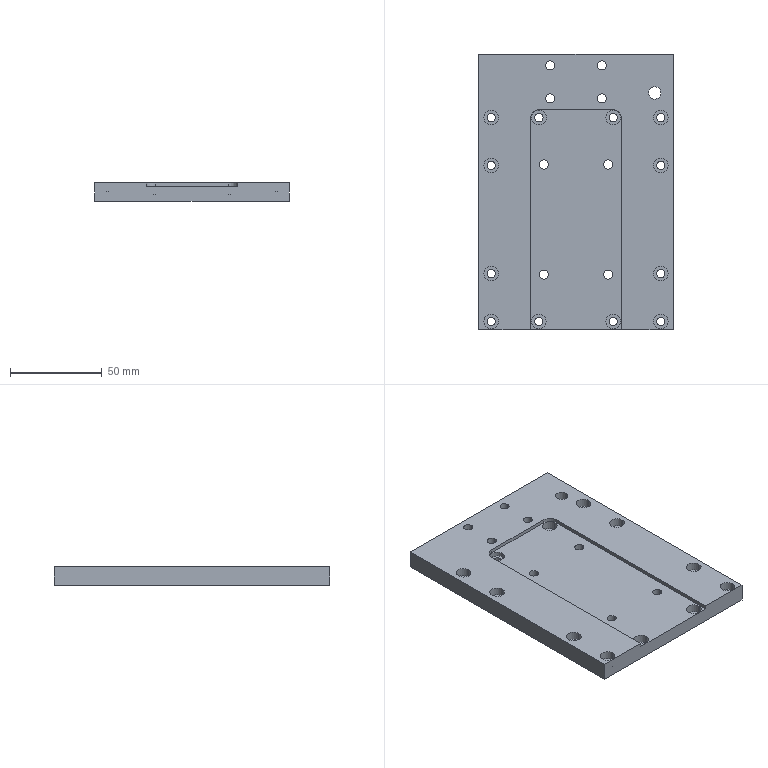Part | STEP file | X77-04014 | 1 solid | 90 faces | box 105.8 x 150 x 10 mm | volume 141335 mm3 | cylinder 68 | plane 22 | commonest cylinder face diameters 4.5 x24 8 x24 5 x16 6.8 x2 10 x2